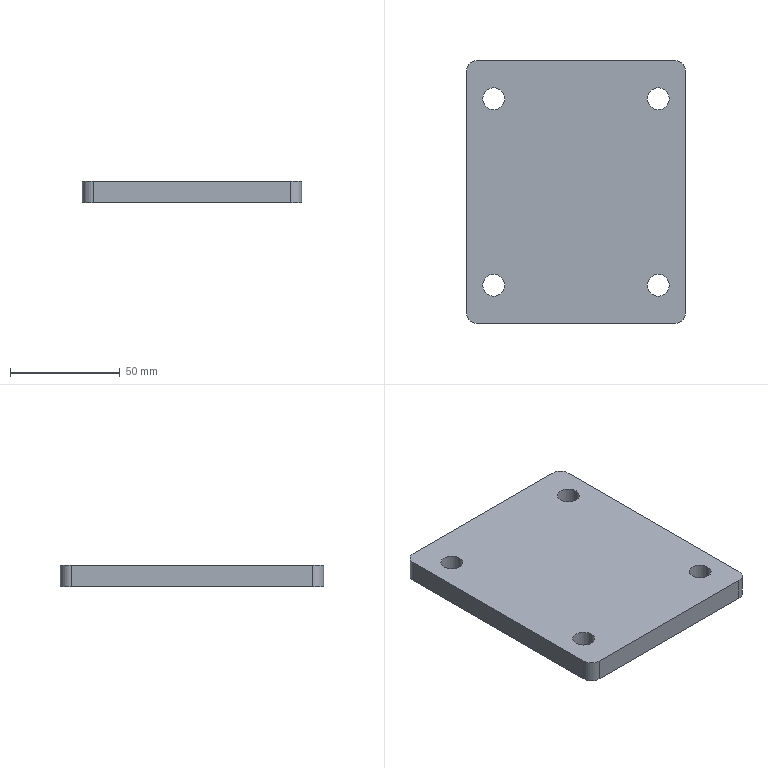Part | SolidWorks | features Extrusion 1 | 1 solid | 18 faces | box 100 x 120 x 10 mm | volume 116644 mm3 | cylinder 12 | plane 6 | commonest cylinder face diameters 10 x12
STEP:
#1=CARTESIAN_POINT('',(7.5,-102.5,10.));
#2=VERTEX_POINT('',#1);
#3=CARTESIAN_POINT('',(17.5,-102.5,10.));
#4=VERTEX_POINT('',#3);
#5=CARTESIAN_POINT('',(12.5,-102.5,10.));
#6=DIRECTION('',(0.,0.,1.));
#7=DIRECTION('',(1.,0.,0.));
#8=AXIS2_PLACEMENT_3D('',#5,#6,#7);
#9=CIRCLE('',#8,5.);
#10=EDGE_CURVE('',#2,#4,#9,.T.);
#11=ORIENTED_EDGE('',*,*,#10,.T.);
#12=CARTESIAN_POINT('',(17.5,-102.5,0.));
#13=VERTEX_POINT('',#12);
#14=CARTESIAN_POINT('',(17.5,-102.5,10.));
#15=DIRECTION('',(0.,0.,-1.));
#16=VECTOR('',#15,1000.);
#17=LINE('',#14,#16);
#18=EDGE_CURVE('',#4,#13,#17,.T.);
#19=ORIENTED_EDGE('',*,*,#18,.T.);
#20=CARTESIAN_POINT('',(7.5,-102.5,0.));
#21=VERTEX_POINT('',#20);
#22=CARTESIAN_POINT('',(12.5,-102.5,0.));
#23=DIRECTION('',(0.,0.,1.));
#24=DIRECTION('',(1.,0.,0.));
#25=AXIS2_PLACEMENT_3D('',#22,#23,#24);
#26=CIRCLE('',#25,5.);
#27=EDGE_CURVE('',#21,#13,#26,.T.);
#28=ORIENTED_EDGE('',*,*,#27,.F.);
#29=CARTESIAN_POINT('',(7.5,-102.5,10.));
#30=DIRECTION('',(0.,0.,-1.));
#31=VECTOR('',#30,1000.);
#32=LINE('',#29,#31);
#33=EDGE_CURVE('',#2,#21,#32,.T.);
#34=ORIENTED_EDGE('',*,*,#33,.F.);
#35=EDGE_LOOP('',(#11,#19,#28,#34));
#36=FACE_OUTER_BOUND('',#35,.T.);
#37=CARTESIAN_POINT('',(12.5,-102.5,10.));
#38=DIRECTION('',(0.,0.,-1.));
#39=DIRECTION('',(-1.,0.,0.));
#40=AXIS2_PLACEMENT_3D('',#37,#38,#39);
#41=CYLINDRICAL_SURFACE('',#40,5.);
#42=ADVANCED_FACE('',(#36),#41,.F.);
#43=CARTESIAN_POINT('',(82.5,-102.5,10.));
#44=VERTEX_POINT('',#43);
#45=CARTESIAN_POINT('',(92.5,-102.5,10.));
#46=VERTEX_POINT('',#45);
#47=CARTESIAN_POINT('',(87.5,-102.5,10.));
#48=DIRECTION('',(0.,0.,1.));
#49=DIRECTION('',(1.,0.,0.));
#50=AXIS2_PLACEMENT_3D('',#47,#48,#49);
#51=CIRCLE('',#50,5.);
#52=EDGE_CURVE('',#44,#46,#51,.T.);
#53=ORIENTED_EDGE('',*,*,#52,.T.);
#54=CARTESIAN_POINT('',(92.5,-102.5,0.));
#55=VERTEX_POINT('',#54);
#56=CARTESIAN_POINT('',(92.5,-102.5,10.));
#57=DIRECTION('',(0.,0.,-1.));
#58=VECTOR('',#57,1000.);
#59=LINE('',#56,#58);
#60=EDGE_CURVE('',#46,#55,#59,.T.);
#61=ORIENTED_EDGE('',*,*,#60,.T.);
#62=CARTESIAN_POINT('',(82.5,-102.5,0.));
#63=VERTEX_POINT('',#62);
#64=CARTESIAN_POINT('',(87.5,-102.5,0.));
#65=DIRECTION('',(0.,0.,1.));
#66=DIRECTION('',(1.,0.,0.));
#67=AXIS2_PLACEMENT_3D('',#64,#65,#66);
#68=CIRCLE('',#67,5.);
#69=EDGE_CURVE('',#63,#55,#68,.T.);
#70=ORIENTED_EDGE('',*,*,#69,.F.);
#71=CARTESIAN_POINT('',(82.5,-102.5,10.));
#72=DIRECTION('',(0.,0.,-1.));
#73=VECTOR('',#72,1000.);
#74=LINE('',#71,#73);
#75=EDGE_CURVE('',#44,#63,#74,.T.);
#76=ORIENTED_EDGE('',*,*,#75,.F.);
#77=EDGE_LOOP('',(#53,#61,#70,#76));
#78=FACE_OUTER_BOUND('',#77,.T.);
#79=CARTESIAN_POINT('',(87.5,-102.5,10.));
#80=DIRECTION('',(0.,0.,-1.));
#81=DIRECTION('',(-1.,0.,0.));
#82=AXIS2_PLACEMENT_3D('',#79,#80,#81);
#83=CYLINDRICAL_SURFACE('',#82,5.);
#84=ADVANCED_FACE('',(#78),#83,.F.);
#85=CARTESIAN_POINT('',(82.5,-17.5,10.));
#86=VERTEX_POINT('',#85);
#87=CARTESIAN_POINT('',(92.5,-17.5,10.));
#88=VERTEX_POINT('',#87);
#89=CARTESIAN_POINT('',(87.5,-17.5,10.));
#90=DIRECTION('',(0.,0.,1.));
#91=DIRECTION('',(1.,0.,0.));
#92=AXIS2_PLACEMENT_3D('',#89,#90,#91);
#93=CIRCLE('',#92,5.);
#94=EDGE_CURVE('',#86,#88,#93,.T.);
#95=ORIENTED_EDGE('',*,*,#94,.T.);
#96=CARTESIAN_POINT('',(92.5,-17.5,0.));
#97=VERTEX_POINT('',#96);
#98=CARTESIAN_POINT('',(92.5,-17.5,10.));
#99=DIRECTION('',(0.,0.,-1.));
#100=VECTOR('',#99,1000.);
#101=LINE('',#98,#100);
#102=EDGE_CURVE('',#88,#97,#101,.T.);
#103=ORIENTED_EDGE('',*,*,#102,.T.);
#104=CARTESIAN_POINT('',(82.5,-17.5,0.));
#105=VERTEX_POINT('',#104);
#106=CARTESIAN_POINT('',(87.5,-17.5,0.));
#107=DIRECTION('',(0.,0.,1.));
#108=DIRECTION('',(1.,0.,0.));
#109=AXIS2_PLACEMENT_3D('',#106,#107,#108);
#110=CIRCLE('',#109,5.);
#111=EDGE_CURVE('',#105,#97,#110,.T.);
#112=ORIENTED_EDGE('',*,*,#111,.F.);
#113=CARTESIAN_POINT('',(82.5,-17.5,10.));
#114=DIRECTION('',(0.,0.,-1.));
#115=VECTOR('',#114,1000.);
#116=LINE('',#113,#115);
#117=EDGE_CURVE('',#86,#105,#116,.T.);
#118=ORIENTED_EDGE('',*,*,#117,.F.);
#119=EDGE_LOOP('',(#95,#103,#112,#118));
#120=FACE_OUTER_BOUND('',#119,.T.);
#121=CARTESIAN_POINT('',(87.5,-17.5,10.));
#122=DIRECTION('',(0.,0.,-1.));
#123=DIRECTION('',(-1.,0.,0.));
#124=AXIS2_PLACEMENT_3D('',#121,#122,#123);
#125=CYLINDRICAL_SURFACE('',#124,5.);
#126=ADVANCED_FACE('',(#120),#125,.F.);
#127=CARTESIAN_POINT('',(7.5,-17.5,10.));
#128=VERTEX_POINT('',#127);
#129=CARTESIAN_POINT('',(17.5,-17.5,10.));
#130=VERTEX_POINT('',#129);
#131=CARTESIAN_POINT('',(12.5,-17.5,10.));
#132=DIRECTION('',(0.,0.,1.));
#133=DIRECTION('',(1.,0.,0.));
#134=AXIS2_PLACEMENT_3D('',#131,#132,#133);
#135=CIRCLE('',#134,5.);
#136=EDGE_CURVE('',#128,#130,#135,.T.);
#137=ORIENTED_EDGE('',*,*,#136,.T.);
#138=CARTESIAN_POINT('',(17.5,-17.5,0.));
#139=VERTEX_POINT('',#138);
#140=CARTESIAN_POINT('',(17.5,-17.5,10.));
#141=DIRECTION('',(0.,0.,-1.));
#142=VECTOR('',#141,1000.);
#143=LINE('',#140,#142);
#144=EDGE_CURVE('',#130,#139,#143,.T.);
#145=ORIENTED_EDGE('',*,*,#144,.T.);
#146=CARTESIAN_POINT('',(7.5,-17.5,0.));
#147=VERTEX_POINT('',#146);
#148=CARTESIAN_POINT('',(12.5,-17.5,0.));
#149=DIRECTION('',(0.,0.,1.));
#150=DIRECTION('',(1.,0.,0.));
#151=AXIS2_PLACEMENT_3D('',#148,#149,#150);
#152=CIRCLE('',#151,5.);
#153=EDGE_CURVE('',#147,#139,#152,.T.);
#154=ORIENTED_EDGE('',*,*,#153,.F.);
#155=CARTESIAN_POINT('',(7.5,-17.5,10.));
#156=DIRECTION('',(0.,0.,-1.));
#157=VECTOR('',#156,1000.);
#158=LINE('',#155,#157);
#159=EDGE_CURVE('',#128,#147,#158,.T.);
#160=ORIENTED_EDGE('',*,*,#159,.F.);
#161=EDGE_LOOP('',(#137,#145,#154,#160));
#162=FACE_OUTER_BOUND('',#161,.T.);
#163=CARTESIAN_POINT('',(12.5,-17.5,10.));
#164=DIRECTION('',(0.,0.,-1.));
#165=DIRECTION('',(-1.,0.,0.));
#166=AXIS2_PLACEMENT_3D('',#163,#164,#165);
#167=CYLINDRICAL_SURFACE('',#166,5.);
#168=ADVANCED_FACE('',(#162),#167,.F.);
#169=ORIENTED_EDGE('',*,*,#52,.F.);
#170=CARTESIAN_POINT('',(87.5,-102.5,10.));
#171=DIRECTION('',(0.,0.,1.));
#172=DIRECTION('',(1.,0.,0.));
#173=AXIS2_PLACEMENT_3D('',#170,#171,#172);
#174=CIRCLE('',#173,5.);
#175=EDGE_CURVE('',#46,#44,#174,.T.);
#176=ORIENTED_EDGE('',*,*,#175,.F.);
#177=EDGE_LOOP('',(#169,#176));
#178=FACE_BOUND('',#177,.T.);
#179=ORIENTED_EDGE('',*,*,#136,.F.);
#180=CARTESIAN_POINT('',(12.5,-17.5,10.));
#181=DIRECTION('',(0.,0.,1.));
#182=DIRECTION('',(1.,0.,0.));
#183=AXIS2_PLACEMENT_3D('',#180,#181,#182);
#184=CIRCLE('',#183,5.);
#185=EDGE_CURVE('',#130,#128,#184,.T.);
#186=ORIENTED_EDGE('',*,*,#185,.F.);
#187=EDGE_LOOP('',(#179,#186));
#188=FACE_BOUND('',#187,.T.);
#189=CARTESIAN_POINT('',(0.,-115.,10.));
#190=VERTEX_POINT('',#189);
#191=CARTESIAN_POINT('',(5.,-120.,10.));
#192=VERTEX_POINT('',#191);
#193=CARTESIAN_POINT('',(5.,-115.,10.));
#194=DIRECTION('',(0.,0.,1.));
#195=DIRECTION('',(1.,0.,0.));
#196=AXIS2_PLACEMENT_3D('',#193,#194,#195);
#197=CIRCLE('',#196,5.);
#198=EDGE_CURVE('',#190,#192,#197,.T.);
#199=ORIENTED_EDGE('',*,*,#198,.T.);
#200=CARTESIAN_POINT('',(95.,-120.,10.));
#201=VERTEX_POINT('',#200);
#202=CARTESIAN_POINT('',(5.,-120.,10.));
#203=DIRECTION('',(1.,0.,0.));
#204=VECTOR('',#203,1000.);
#205=LINE('',#202,#204);
#206=EDGE_CURVE('',#192,#201,#205,.T.);
#207=ORIENTED_EDGE('',*,*,#206,.T.);
#208=CARTESIAN_POINT('',(100.,-115.,10.));
#209=VERTEX_POINT('',#208);
#210=CARTESIAN_POINT('',(95.,-115.,10.));
#211=DIRECTION('',(0.,0.,1.));
#212=DIRECTION('',(1.,0.,0.));
#213=AXIS2_PLACEMENT_3D('',#210,#211,#212);
#214=CIRCLE('',#213,5.);
#215=EDGE_CURVE('',#201,#209,#214,.T.);
#216=ORIENTED_EDGE('',*,*,#215,.T.);
#217=CARTESIAN_POINT('',(100.,-5.,10.));
#218=VERTEX_POINT('',#217);
#219=CARTESIAN_POINT('',(100.,-5.,10.));
#220=DIRECTION('',(0.,1.,0.));
#221=VECTOR('',#220,1000.);
#222=LINE('',#219,#221);
#223=EDGE_CURVE('',#209,#218,#222,.T.);
#224=ORIENTED_EDGE('',*,*,#223,.T.);
#225=CARTESIAN_POINT('',(95.,0.,10.));
#226=VERTEX_POINT('',#225);
#227=CARTESIAN_POINT('',(95.,-5.,10.));
#228=DIRECTION('',(0.,0.,1.));
#229=DIRECTION('',(1.,0.,0.));
#230=AXIS2_PLACEMENT_3D('',#227,#228,#229);
#231=CIRCLE('',#230,5.);
#232=EDGE_CURVE('',#218,#226,#231,.T.);
#233=ORIENTED_EDGE('',*,*,#232,.T.);
#234=CARTESIAN_POINT('',(5.,0.,10.));
#235=VERTEX_POINT('',#234);
#236=CARTESIAN_POINT('',(5.,0.,10.));
#237=DIRECTION('',(-1.,0.,0.));
#238=VECTOR('',#237,1000.);
#239=LINE('',#236,#238);
#240=EDGE_CURVE('',#226,#235,#239,.T.);
#241=ORIENTED_EDGE('',*,*,#240,.T.);
#242=CARTESIAN_POINT('',(0.,-5.,10.));
#243=VERTEX_POINT('',#242);
#244=CARTESIAN_POINT('',(5.,-5.,10.));
#245=DIRECTION('',(0.,0.,1.));
#246=DIRECTION('',(-1.,0.,0.));
#247=AXIS2_PLACEMENT_3D('',#244,#245,#246);
#248=CIRCLE('',#247,5.);
#249=EDGE_CURVE('',#235,#243,#248,.T.);
#250=ORIENTED_EDGE('',*,*,#249,.T.);
#251=CARTESIAN_POINT('',(0.,-5.,10.));
#252=DIRECTION('',(0.,-1.,0.));
#253=VECTOR('',#252,1000.);
#254=LINE('',#251,#253);
#255=EDGE_CURVE('',#243,#190,#254,.T.);
#256=ORIENTED_EDGE('',*,*,#255,.T.);
#257=EDGE_LOOP('',(#199,#207,#216,#224,#233,#241,#250,#256));
#258=FACE_OUTER_BOUND('',#257,.T.);
#259=ORIENTED_EDGE('',*,*,#94,.F.);
#260=CARTESIAN_POINT('',(87.5,-17.5,10.));
#261=DIRECTION('',(0.,0.,1.));
#262=DIRECTION('',(1.,0.,0.));
#263=AXIS2_PLACEMENT_3D('',#260,#261,#262);
#264=CIRCLE('',#263,5.);
#265=EDGE_CURVE('',#88,#86,#264,.T.);
#266=ORIENTED_EDGE('',*,*,#265,.F.);
#267=EDGE_LOOP('',(#259,#266));
#268=FACE_BOUND('',#267,.T.);
#269=ORIENTED_EDGE('',*,*,#10,.F.);
#270=CARTESIAN_POINT('',(12.5,-102.5,10.));
#271=DIRECTION('',(0.,0.,1.));
#272=DIRECTION('',(1.,0.,0.));
#273=AXIS2_PLACEMENT_3D('',#270,#271,#272);
#274=CIRCLE('',#273,5.);
#275=EDGE_CURVE('',#4,#2,#274,.T.);
#276=ORIENTED_EDGE('',*,*,#275,.F.);
#277=EDGE_LOOP('',(#269,#276));
#278=FACE_BOUND('',#277,.T.);
#279=CARTESIAN_POINT('',(5.,-115.,10.));
#280=DIRECTION('',(0.,0.,1.));
#281=DIRECTION('',(1.,0.,0.));
#282=AXIS2_PLACEMENT_3D('',#279,#280,#281);
#283=PLANE('',#282);
#284=ADVANCED_FACE('',(#178,#188,#258,#268,#278),#283,.T.);
#285=CARTESIAN_POINT('',(0.,-115.,0.));
#286=VERTEX_POINT('',#285);
#287=CARTESIAN_POINT('',(5.,-120.,0.));
#288=VERTEX_POINT('',#287);
#289=CARTESIAN_POINT('',(5.,-115.,0.));
#290=DIRECTION('',(0.,0.,1.));
#291=DIRECTION('',(1.,0.,0.));
#292=AXIS2_PLACEMENT_3D('',#289,#290,#291);
#293=CIRCLE('',#292,5.);
#294=EDGE_CURVE('',#286,#288,#293,.T.);
#295=ORIENTED_EDGE('',*,*,#294,.F.);
#296=CARTESIAN_POINT('',(0.,-5.,0.));
#297=VERTEX_POINT('',#296);
#298=CARTESIAN_POINT('',(0.,-5.,0.));
#299=DIRECTION('',(0.,-1.,0.));
#300=VECTOR('',#299,1000.);
#301=LINE('',#298,#300);
#302=EDGE_CURVE('',#297,#286,#301,.T.);
#303=ORIENTED_EDGE('',*,*,#302,.F.);
#304=CARTESIAN_POINT('',(5.,0.,0.));
#305=VERTEX_POINT('',#304);
#306=CARTESIAN_POINT('',(5.,-5.,0.));
#307=DIRECTION('',(0.,0.,1.));
#308=DIRECTION('',(-1.,0.,0.));
#309=AXIS2_PLACEMENT_3D('',#306,#307,#308);
#310=CIRCLE('',#309,5.);
#311=EDGE_CURVE('',#305,#297,#310,.T.);
#312=ORIENTED_EDGE('',*,*,#311,.F.);
#313=CARTESIAN_POINT('',(95.,0.,0.));
#314=VERTEX_POINT('',#313);
#315=CARTESIAN_POINT('',(5.,0.,0.));
#316=DIRECTION('',(-1.,0.,0.));
#317=VECTOR('',#316,1000.);
#318=LINE('',#315,#317);
#319=EDGE_CURVE('',#314,#305,#318,.T.);
#320=ORIENTED_EDGE('',*,*,#319,.F.);
#321=CARTESIAN_POINT('',(100.,-5.,0.));
#322=VERTEX_POINT('',#321);
#323=CARTESIAN_POINT('',(95.,-5.,0.));
#324=DIRECTION('',(0.,0.,1.));
#325=DIRECTION('',(1.,0.,0.));
#326=AXIS2_PLACEMENT_3D('',#323,#324,#325);
#327=CIRCLE('',#326,5.);
#328=EDGE_CURVE('',#322,#314,#327,.T.);
#329=ORIENTED_EDGE('',*,*,#328,.F.);
#330=CARTESIAN_POINT('',(100.,-115.,0.));
#331=VERTEX_POINT('',#330);
#332=CARTESIAN_POINT('',(100.,-5.,0.));
#333=DIRECTION('',(0.,1.,0.));
#334=VECTOR('',#333,1000.);
#335=LINE('',#332,#334);
#336=EDGE_CURVE('',#331,#322,#335,.T.);
#337=ORIENTED_EDGE('',*,*,#336,.F.);
#338=CARTESIAN_POINT('',(95.,-120.,0.));
#339=VERTEX_POINT('',#338);
#340=CARTESIAN_POINT('',(95.,-115.,0.));
#341=DIRECTION('',(0.,0.,1.));
#342=DIRECTION('',(1.,0.,0.));
#343=AXIS2_PLACEMENT_3D('',#340,#341,#342);
#344=CIRCLE('',#343,5.);
#345=EDGE_CURVE('',#339,#331,#344,.T.);
#346=ORIENTED_EDGE('',*,*,#345,.F.);
#347=CARTESIAN_POINT('',(5.,-120.,0.));
#348=DIRECTION('',(1.,0.,0.));
#349=VECTOR('',#348,1000.);
#350=LINE('',#347,#349);
#351=EDGE_CURVE('',#288,#339,#350,.T.);
#352=ORIENTED_EDGE('',*,*,#351,.F.);
#353=EDGE_LOOP('',(#295,#303,#312,#320,#329,#337,#346,#352));
#354=FACE_OUTER_BOUND('',#353,.T.);
#355=ORIENTED_EDGE('',*,*,#153,.T.);
#356=CARTESIAN_POINT('',(12.5,-17.5,0.));
#357=DIRECTION('',(0.,0.,1.));
#358=DIRECTION('',(1.,0.,0.));
#359=AXIS2_PLACEMENT_3D('',#356,#357,#358);
#360=CIRCLE('',#359,5.);
#361=EDGE_CURVE('',#139,#147,#360,.T.);
#362=ORIENTED_EDGE('',*,*,#361,.T.);
#363=EDGE_LOOP('',(#355,#362));
#364=FACE_BOUND('',#363,.T.);
#365=ORIENTED_EDGE('',*,*,#111,.T.);
#366=CARTESIAN_POINT('',(87.5,-17.5,0.));
#367=DIRECTION('',(0.,0.,1.));
#368=DIRECTION('',(1.,0.,0.));
#369=AXIS2_PLACEMENT_3D('',#366,#367,#368);
#370=CIRCLE('',#369,5.);
#371=EDGE_CURVE('',#97,#105,#370,.T.);
#372=ORIENTED_EDGE('',*,*,#371,.T.);
#373=EDGE_LOOP('',(#365,#372));
#374=FACE_BOUND('',#373,.T.);
#375=ORIENTED_EDGE('',*,*,#69,.T.);
#376=CARTESIAN_POINT('',(87.5,-102.5,0.));
#377=DIRECTION('',(0.,0.,1.));
#378=DIRECTION('',(1.,0.,0.));
#379=AXIS2_PLACEMENT_3D('',#376,#377,#378);
#380=CIRCLE('',#379,5.);
#381=EDGE_CURVE('',#55,#63,#380,.T.);
#382=ORIENTED_EDGE('',*,*,#381,.T.);
#383=EDGE_LOOP('',(#375,#382));
#384=FACE_BOUND('',#383,.T.);
#385=ORIENTED_EDGE('',*,*,#27,.T.);
#386=CARTESIAN_POINT('',(12.5,-102.5,0.));
#387=DIRECTION('',(0.,0.,1.));
#388=DIRECTION('',(1.,0.,0.));
#389=AXIS2_PLACEMENT_3D('',#386,#387,#388);
#390=CIRCLE('',#389,5.);
#391=EDGE_CURVE('',#13,#21,#390,.T.);
#392=ORIENTED_EDGE('',*,*,#391,.T.);
#393=EDGE_LOOP('',(#385,#392));
#394=FACE_BOUND('',#393,.T.);
#395=CARTESIAN_POINT('',(5.,-115.,0.));
#396=DIRECTION('',(0.,0.,1.));
#397=DIRECTION('',(1.,0.,0.));
#398=AXIS2_PLACEMENT_3D('',#395,#396,#397);
#399=PLANE('',#398);
#400=ADVANCED_FACE('',(#354,#364,#374,#384,#394),#399,.F.);
#401=ORIENTED_EDGE('',*,*,#294,.T.);
#402=CARTESIAN_POINT('',(5.,-120.,10.));
#403=DIRECTION('',(0.,0.,-1.));
#404=VECTOR('',#403,1000.);
#405=LINE('',#402,#404);
#406=EDGE_CURVE('',#192,#288,#405,.T.);
#407=ORIENTED_EDGE('',*,*,#406,.F.);
#408=ORIENTED_EDGE('',*,*,#198,.F.);
#409=CARTESIAN_POINT('',(0.,-115.,10.));
#410=DIRECTION('',(0.,0.,-1.));
#411=VECTOR('',#410,1000.);
#412=LINE('',#409,#411);
#413=EDGE_CURVE('',#190,#286,#412,.T.);
#414=ORIENTED_EDGE('',*,*,#413,.T.);
#415=EDGE_LOOP('',(#401,#407,#408,#414));
#416=FACE_OUTER_BOUND('',#415,.T.);
#417=CARTESIAN_POINT('',(5.,-115.,10.));
#418=DIRECTION('',(0.,0.,-1.));
#419=DIRECTION('',(-1.,0.,0.));
#420=AXIS2_PLACEMENT_3D('',#417,#418,#419);
#421=CYLINDRICAL_SURFACE('',#420,5.);
#422=ADVANCED_FACE('',(#416),#421,.T.);
#423=ORIENTED_EDGE('',*,*,#351,.T.);
#424=CARTESIAN_POINT('',(95.,-120.,10.));
#425=DIRECTION('',(0.,0.,-1.));
#426=VECTOR('',#425,1000.);
#427=LINE('',#424,#426);
#428=EDGE_CURVE('',#201,#339,#427,.T.);
#429=ORIENTED_EDGE('',*,*,#428,.F.);
#430=ORIENTED_EDGE('',*,*,#206,.F.);
#431=ORIENTED_EDGE('',*,*,#406,.T.);
#432=EDGE_LOOP('',(#423,#429,#430,#431));
#433=FACE_OUTER_BOUND('',#432,.T.);
#434=CARTESIAN_POINT('',(5.,-120.,10.));
#435=DIRECTION('',(0.,1.,0.));
#436=DIRECTION('',(0.,0.,1.));
#437=AXIS2_PLACEMENT_3D('',#434,#435,#436);
#438=PLANE('',#437);
#439=ADVANCED_FACE('',(#433),#438,.F.);
#440=ORIENTED_EDGE('',*,*,#345,.T.);
#441=CARTESIAN_POINT('',(100.,-115.,10.));
#442=DIRECTION('',(0.,0.,-1.));
#443=VECTOR('',#442,1000.);
#444=LINE('',#441,#443);
#445=EDGE_CURVE('',#209,#331,#444,.T.);
#446=ORIENTED_EDGE('',*,*,#445,.F.);
#447=ORIENTED_EDGE('',*,*,#215,.F.);
#448=ORIENTED_EDGE('',*,*,#428,.T.);
#449=EDGE_LOOP('',(#440,#446,#447,#448));
#450=FACE_OUTER_BOUND('',#449,.T.);
#451=CARTESIAN_POINT('',(95.,-115.,10.));
#452=DIRECTION('',(0.,0.,-1.));
#453=DIRECTION('',(-1.,0.,0.));
#454=AXIS2_PLACEMENT_3D('',#451,#452,#453);
#455=CYLINDRICAL_SURFACE('',#454,5.);
#456=ADVANCED_FACE('',(#450),#455,.T.);
#457=ORIENTED_EDGE('',*,*,#336,.T.);
#458=CARTESIAN_POINT('',(100.,-5.,10.));
#459=DIRECTION('',(0.,0.,-1.));
#460=VECTOR('',#459,1000.);
#461=LINE('',#458,#460);
#462=EDGE_CURVE('',#218,#322,#461,.T.);
#463=ORIENTED_EDGE('',*,*,#462,.F.);
#464=ORIENTED_EDGE('',*,*,#223,.F.);
#465=ORIENTED_EDGE('',*,*,#445,.T.);
#466=EDGE_LOOP('',(#457,#463,#464,#465));
#467=FACE_OUTER_BOUND('',#466,.T.);
#468=CARTESIAN_POINT('',(100.,-5.,10.));
#469=DIRECTION('',(-1.,0.,0.));
#470=DIRECTION('',(0.,-1.,0.));
#471=AXIS2_PLACEMENT_3D('',#468,#469,#470);
#472=PLANE('',#471);
#473=ADVANCED_FACE('',(#467),#472,.F.);
#474=ORIENTED_EDGE('',*,*,#328,.T.);
#475=CARTESIAN_POINT('',(95.,0.,10.));
#476=DIRECTION('',(0.,0.,-1.));
#477=VECTOR('',#476,1000.);
#478=LINE('',#475,#477);
#479=EDGE_CURVE('',#226,#314,#478,.T.);
#480=ORIENTED_EDGE('',*,*,#479,.F.);
#481=ORIENTED_EDGE('',*,*,#232,.F.);
#482=ORIENTED_EDGE('',*,*,#462,.T.);
#483=EDGE_LOOP('',(#474,#480,#481,#482));
#484=FACE_OUTER_BOUND('',#483,.T.);
#485=CARTESIAN_POINT('',(95.,-5.,10.));
#486=DIRECTION('',(0.,0.,-1.));
#487=DIRECTION('',(-1.,0.,0.));
#488=AXIS2_PLACEMENT_3D('',#485,#486,#487);
#489=CYLINDRICAL_SURFACE('',#488,5.);
#490=ADVANCED_FACE('',(#484),#489,.T.);
#491=ORIENTED_EDGE('',*,*,#319,.T.);
#492=CARTESIAN_POINT('',(5.,0.,10.));
#493=DIRECTION('',(0.,0.,-1.));
#494=VECTOR('',#493,1000.);
#495=LINE('',#492,#494);
#496=EDGE_CURVE('',#235,#305,#495,.T.);
#497=ORIENTED_EDGE('',*,*,#496,.F.);
#498=ORIENTED_EDGE('',*,*,#240,.F.);
#499=ORIENTED_EDGE('',*,*,#479,.T.);
#500=EDGE_LOOP('',(#491,#497,#498,#499));
#501=FACE_OUTER_BOUND('',#500,.T.);
#502=CARTESIAN_POINT('',(5.,0.,10.));
#503=DIRECTION('',(0.,-1.,0.));
#504=DIRECTION('',(0.,0.,-1.));
#505=AXIS2_PLACEMENT_3D('',#502,#503,#504);
#506=PLANE('',#505);
#507=ADVANCED_FACE('',(#501),#506,.F.);
#508=ORIENTED_EDGE('',*,*,#311,.T.);
#509=CARTESIAN_POINT('',(0.,-5.,10.));
#510=DIRECTION('',(0.,0.,-1.));
#511=VECTOR('',#510,1000.);
#512=LINE('',#509,#511);
#513=EDGE_CURVE('',#243,#297,#512,.T.);
#514=ORIENTED_EDGE('',*,*,#513,.F.);
#515=ORIENTED_EDGE('',*,*,#249,.F.);
#516=ORIENTED_EDGE('',*,*,#496,.T.);
#517=EDGE_LOOP('',(#508,#514,#515,#516));
#518=FACE_OUTER_BOUND('',#517,.T.);
#519=CARTESIAN_POINT('',(5.,-5.,10.));
#520=DIRECTION('',(0.,0.,-1.));
#521=DIRECTION('',(-1.,0.,0.));
#522=AXIS2_PLACEMENT_3D('',#519,#520,#521);
#523=CYLINDRICAL_SURFACE('',#522,5.);
#524=ADVANCED_FACE('',(#518),#523,.T.);
#525=ORIENTED_EDGE('',*,*,#302,.T.);
#526=ORIENTED_EDGE('',*,*,#413,.F.);
#527=ORIENTED_EDGE('',*,*,#255,.F.);
#528=ORIENTED_EDGE('',*,*,#513,.T.);
#529=EDGE_LOOP('',(#525,#526,#527,#528));
#530=FACE_OUTER_BOUND('',#529,.T.);
#531=CARTESIAN_POINT('',(0.,-5.,10.));
#532=DIRECTION('',(1.,0.,0.));
#533=DIRECTION('',(0.,1.,0.));
#534=AXIS2_PLACEMENT_3D('',#531,#532,#533);
#535=PLANE('',#534);
#536=ADVANCED_FACE('',(#530),#535,.F.);
#537=ORIENTED_EDGE('',*,*,#144,.F.);
#538=ORIENTED_EDGE('',*,*,#185,.T.);
#539=ORIENTED_EDGE('',*,*,#159,.T.);
#540=ORIENTED_EDGE('',*,*,#361,.F.);
#541=EDGE_LOOP('',(#537,#538,#539,#540));
#542=FACE_OUTER_BOUND('',#541,.T.);
#543=CARTESIAN_POINT('',(12.5,-17.5,10.));
#544=DIRECTION('',(0.,0.,-1.));
#545=DIRECTION('',(-1.,0.,0.));
#546=AXIS2_PLACEMENT_3D('',#543,#544,#545);
#547=CYLINDRICAL_SURFACE('',#546,5.);
#548=ADVANCED_FACE('',(#542),#547,.F.);
#549=ORIENTED_EDGE('',*,*,#102,.F.);
#550=ORIENTED_EDGE('',*,*,#265,.T.);
#551=ORIENTED_EDGE('',*,*,#117,.T.);
#552=ORIENTED_EDGE('',*,*,#371,.F.);
#553=EDGE_LOOP('',(#549,#550,#551,#552));
#554=FACE_OUTER_BOUND('',#553,.T.);
#555=CARTESIAN_POINT('',(87.5,-17.5,10.));
#556=DIRECTION('',(0.,0.,-1.));
#557=DIRECTION('',(-1.,0.,0.));
#558=AXIS2_PLACEMENT_3D('',#555,#556,#557);
#559=CYLINDRICAL_SURFACE('',#558,5.);
#560=ADVANCED_FACE('',(#554),#559,.F.);
#561=ORIENTED_EDGE('',*,*,#60,.F.);
#562=ORIENTED_EDGE('',*,*,#175,.T.);
#563=ORIENTED_EDGE('',*,*,#75,.T.);
#564=ORIENTED_EDGE('',*,*,#381,.F.);
#565=EDGE_LOOP('',(#561,#562,#563,#564));
#566=FACE_OUTER_BOUND('',#565,.T.);
#567=CARTESIAN_POINT('',(87.5,-102.5,10.));
#568=DIRECTION('',(0.,0.,-1.));
#569=DIRECTION('',(-1.,0.,0.));
#570=AXIS2_PLACEMENT_3D('',#567,#568,#569);
#571=CYLINDRICAL_SURFACE('',#570,5.);
#572=ADVANCED_FACE('',(#566),#571,.F.);
#573=ORIENTED_EDGE('',*,*,#18,.F.);
#574=ORIENTED_EDGE('',*,*,#275,.T.);
#575=ORIENTED_EDGE('',*,*,#33,.T.);
#576=ORIENTED_EDGE('',*,*,#391,.F.);
#577=EDGE_LOOP('',(#573,#574,#575,#576));
#578=FACE_OUTER_BOUND('',#577,.T.);
#579=CARTESIAN_POINT('',(12.5,-102.5,10.));
#580=DIRECTION('',(0.,0.,-1.));
#581=DIRECTION('',(-1.,0.,0.));
#582=AXIS2_PLACEMENT_3D('',#579,#580,#581);
#583=CYLINDRICAL_SURFACE('',#582,5.);
#584=ADVANCED_FACE('',(#578),#583,.F.);
#585=CLOSED_SHELL('',(#42,#84,#126,#168,#284,#400,#422,#439,#456,#473,#490,#507,#524,#536,#548,#560,#572,#584));
#586=MANIFOLD_SOLID_BREP('',#585);
#587=CARTESIAN_POINT('',(0.,0.,0.));
#588=DIRECTION('',(0.,0.,1.));
#589=DIRECTION('',(1.,0.,0.));
#590=AXIS2_PLACEMENT_3D('',#587,#588,#589);
#591=(LENGTH_UNIT()NAMED_UNIT(*)SI_UNIT(.MILLI.,.METRE.));
#592=UNCERTAINTY_MEASURE_WITH_UNIT(LENGTH_MEASURE(0.00001),#591,'','');
#593=(NAMED_UNIT(*)PLANE_ANGLE_UNIT()SI_UNIT($,.RADIAN.));
#594=(NAMED_UNIT(*)SI_UNIT($,.STERADIAN.)SOLID_ANGLE_UNIT());
#595=(GEOMETRIC_REPRESENTATION_CONTEXT(3)GLOBAL_UNCERTAINTY_ASSIGNED_CONTEXT((#592))GLOBAL_UNIT_ASSIGNED_CONTEXT((#591,#593,#594))REPRESENTATION_CONTEXT('',''));
#596=ADVANCED_BREP_SHAPE_REPRESENTATION('',(#586,#590),#595);